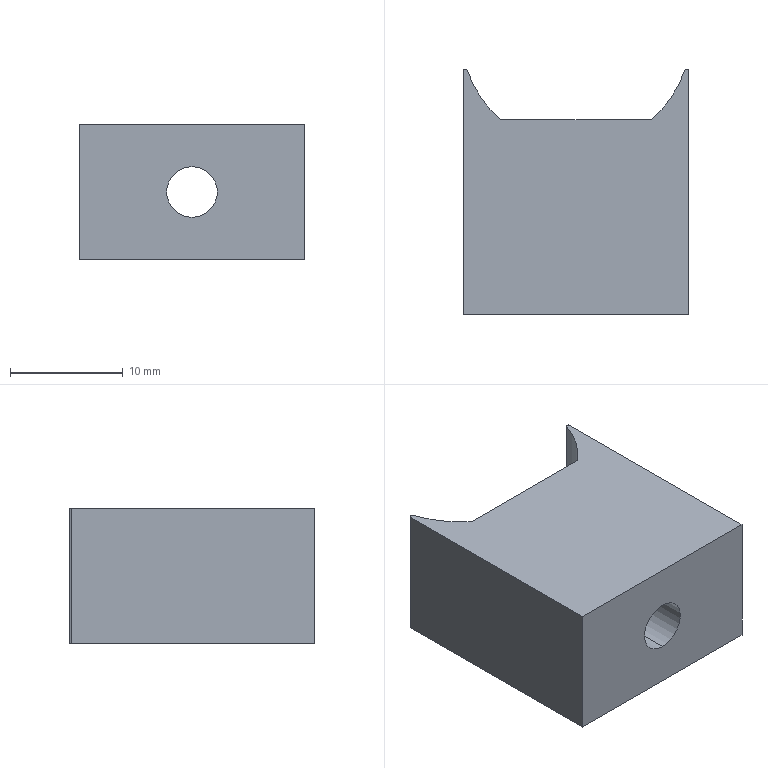Part | STEP file | cylinder positioning fork | 1 solid | 17 faces | box 20 x 21.799 x 12 mm | volume 3903 mm3 | cylinder 10 | plane 7 | commonest cylinder face diameters 0.4 x4 4.5 x2 8 x2 20.4 x2
STEP:
#1=CARTESIAN_POINT('',(0.,0.,0.));
#2=DIRECTION('',(0.,0.,1.));
#3=DIRECTION('',(1.,0.,0.));
#4=AXIS2_PLACEMENT_3D('',#1,#2,#3);
#5=CARTESIAN_POINT('',(0.,-11.7,10.));
#6=VERTEX_POINT('',#5);
#7=CARTESIAN_POINT('',(0.,-7.7,10.));
#8=VERTEX_POINT('',#7);
#9=CARTESIAN_POINT('',(0.,-7.7,10.));
#10=DIRECTION('',(0.,1.,0.));
#11=VECTOR('',#10,1.);
#12=LINE('',#9,#11);
#13=CARTESIAN_POINT('',(0.,-7.7,6.));
#14=DIRECTION('',(0.,1.,0.));
#15=DIRECTION('',(0.,0.,1.));
#16=AXIS2_PLACEMENT_3D('',#13,#14,#15);
#17=CYLINDRICAL_SURFACE('',#16,4.);
#18=CARTESIAN_POINT('',(6.283,0.));
#19=DIRECTION('',(0.,1.));
#20=VECTOR('',#19,1.);
#21=LINE('',#18,#20);
#22=(GEOMETRIC_REPRESENTATION_CONTEXT(2)PARAMETRIC_REPRESENTATION_CONTEXT()REPRESENTATION_CONTEXT('',''));
#23=DEFINITIONAL_REPRESENTATION('',(#21),#22);
#24=PCURVE('',#17,#23);
#25=CARTESIAN_POINT('',(0.,-7.7,6.));
#26=DIRECTION('',(0.,1.,0.));
#27=DIRECTION('',(0.,0.,1.));
#28=AXIS2_PLACEMENT_3D('',#25,#26,#27);
#29=CYLINDRICAL_SURFACE('',#28,4.);
#30=CARTESIAN_POINT('',(0.,0.));
#31=DIRECTION('',(0.,1.));
#32=VECTOR('',#31,1.);
#33=LINE('',#30,#32);
#34=(GEOMETRIC_REPRESENTATION_CONTEXT(2)PARAMETRIC_REPRESENTATION_CONTEXT()REPRESENTATION_CONTEXT('',''));
#35=DEFINITIONAL_REPRESENTATION('',(#33),#34);
#36=PCURVE('',#29,#35);
#37=SURFACE_CURVE('',#12,(#24,#36),.PCURVE_S1.);
#38=EDGE_CURVE('',#6,#8,#37,.T.);
#39=ORIENTED_EDGE('',*,*,#38,.T.);
#40=CARTESIAN_POINT('',(0.,-7.7,2.));
#41=VERTEX_POINT('',#40);
#42=CARTESIAN_POINT('',(0.,-7.7,6.));
#43=DIRECTION('',(0.,1.,0.));
#44=DIRECTION('',(0.,0.,1.));
#45=AXIS2_PLACEMENT_3D('',#42,#43,#44);
#46=CIRCLE('',#45,4.);
#47=CARTESIAN_POINT('',(0.,0.));
#48=DIRECTION('',(1.,0.));
#49=VECTOR('',#48,1.);
#50=LINE('',#47,#49);
#51=(GEOMETRIC_REPRESENTATION_CONTEXT(2)PARAMETRIC_REPRESENTATION_CONTEXT()REPRESENTATION_CONTEXT('',''));
#52=DEFINITIONAL_REPRESENTATION('',(#50),#51);
#53=PCURVE('',#17,#52);
#54=CARTESIAN_POINT('',(-6.69,-7.7,12.));
#55=DIRECTION('',(0.,-1.,0.));
#56=DIRECTION('',(0.,0.,-1.));
#57=AXIS2_PLACEMENT_3D('',#54,#55,#56);
#58=PLANE('',#57);
#59=CARTESIAN_POINT('',(2.,6.69));
#60=CARTESIAN_POINT('',(2.,13.618));
#61=CARTESIAN_POINT('',(8.,10.154));
#62=CARTESIAN_POINT('',(14.,6.69));
#63=CARTESIAN_POINT('',(8.,3.225));
#64=CARTESIAN_POINT('',(2.,-0.2387));
#65=CARTESIAN_POINT('',(2.,6.69));
#66=(BOUNDED_CURVE()B_SPLINE_CURVE(2,(#59,#60,#61,#62,#63,#64,#65),.UNSPECIFIED.,.T.,.F.)B_SPLINE_CURVE_WITH_KNOTS((1,2,2,2,2,1),(-2.094,0.,2.094,4.189,6.283,8.378),.UNSPECIFIED.)CURVE()GEOMETRIC_REPRESENTATION_ITEM()RATIONAL_B_SPLINE_CURVE((1.,0.5,1.,0.5,1.,0.5,1.))REPRESENTATION_ITEM(''));
#67=(GEOMETRIC_REPRESENTATION_CONTEXT(2)PARAMETRIC_REPRESENTATION_CONTEXT()REPRESENTATION_CONTEXT('',''));
#68=DEFINITIONAL_REPRESENTATION('',(#66),#67);
#69=PCURVE('',#58,#68);
#70=SURFACE_CURVE('',#46,(#53,#69),.PCURVE_S1.);
#71=EDGE_CURVE('',#41,#8,#70,.T.);
#72=ORIENTED_EDGE('',*,*,#71,.F.);
#73=CARTESIAN_POINT('',(0.,-11.7,2.));
#74=VERTEX_POINT('',#73);
#75=CARTESIAN_POINT('',(0.,-7.7,2.));
#76=DIRECTION('',(0.,1.,0.));
#77=VECTOR('',#76,1.);
#78=LINE('',#75,#77);
#79=CARTESIAN_POINT('',(3.142,0.));
#80=DIRECTION('',(0.,1.));
#81=VECTOR('',#80,1.);
#82=LINE('',#79,#81);
#83=(GEOMETRIC_REPRESENTATION_CONTEXT(2)PARAMETRIC_REPRESENTATION_CONTEXT()REPRESENTATION_CONTEXT('',''));
#84=DEFINITIONAL_REPRESENTATION('',(#82),#83);
#85=PCURVE('',#17,#84);
#86=CARTESIAN_POINT('',(3.142,0.));
#87=DIRECTION('',(0.,1.));
#88=VECTOR('',#87,1.);
#89=LINE('',#86,#88);
#90=(GEOMETRIC_REPRESENTATION_CONTEXT(2)PARAMETRIC_REPRESENTATION_CONTEXT()REPRESENTATION_CONTEXT('',''));
#91=DEFINITIONAL_REPRESENTATION('',(#89),#90);
#92=PCURVE('',#29,#91);
#93=SURFACE_CURVE('',#78,(#85,#92),.PCURVE_S1.);
#94=EDGE_CURVE('',#74,#41,#93,.T.);
#95=ORIENTED_EDGE('',*,*,#94,.F.);
#96=CARTESIAN_POINT('',(0.,-11.7,6.));
#97=DIRECTION('',(0.,1.,0.));
#98=DIRECTION('',(0.,0.,1.));
#99=AXIS2_PLACEMENT_3D('',#96,#97,#98);
#100=CIRCLE('',#99,4.);
#101=CARTESIAN_POINT('',(0.,-4.));
#102=DIRECTION('',(1.,0.));
#103=VECTOR('',#102,1.);
#104=LINE('',#101,#103);
#105=(GEOMETRIC_REPRESENTATION_CONTEXT(2)PARAMETRIC_REPRESENTATION_CONTEXT()REPRESENTATION_CONTEXT('',''));
#106=DEFINITIONAL_REPRESENTATION('',(#104),#105);
#107=PCURVE('',#17,#106);
#108=CARTESIAN_POINT('',(2.25,-11.7,6.));
#109=DIRECTION('',(0.,-1.,0.));
#110=DIRECTION('',(0.,0.,-1.));
#111=AXIS2_PLACEMENT_3D('',#108,#109,#110);
#112=PLANE('',#111);
#113=CARTESIAN_POINT('',(-4.,-2.25));
#114=CARTESIAN_POINT('',(-4.,4.678));
#115=CARTESIAN_POINT('',(2.,1.214));
#116=CARTESIAN_POINT('',(8.,-2.25));
#117=CARTESIAN_POINT('',(2.,-5.714));
#118=CARTESIAN_POINT('',(-4.,-9.178));
#119=CARTESIAN_POINT('',(-4.,-2.25));
#120=(BOUNDED_CURVE()B_SPLINE_CURVE(2,(#113,#114,#115,#116,#117,#118,#119),.UNSPECIFIED.,.T.,.F.)B_SPLINE_CURVE_WITH_KNOTS((1,2,2,2,2,1),(-2.094,0.,2.094,4.189,6.283,8.378),.UNSPECIFIED.)CURVE()GEOMETRIC_REPRESENTATION_ITEM()RATIONAL_B_SPLINE_CURVE((1.,0.5,1.,0.5,1.,0.5,1.))REPRESENTATION_ITEM(''));
#121=(GEOMETRIC_REPRESENTATION_CONTEXT(2)PARAMETRIC_REPRESENTATION_CONTEXT()REPRESENTATION_CONTEXT('',''));
#122=DEFINITIONAL_REPRESENTATION('',(#120),#121);
#123=PCURVE('',#112,#122);
#124=SURFACE_CURVE('',#100,(#107,#123),.PCURVE_S1.);
#125=EDGE_CURVE('',#74,#6,#124,.T.);
#126=ORIENTED_EDGE('',*,*,#125,.T.);
#127=EDGE_LOOP('',(#39,#72,#95,#126));
#128=FACE_BOUND('',#127,.F.);
#129=ADVANCED_FACE('',(#128),#17,.F.);
#130=CARTESIAN_POINT('',(0.,-25.,8.25));
#131=VERTEX_POINT('',#130);
#132=CARTESIAN_POINT('',(0.,-11.7,8.25));
#133=VERTEX_POINT('',#132);
#134=CARTESIAN_POINT('',(0.,-7.7,8.25));
#135=DIRECTION('',(0.,1.,0.));
#136=VECTOR('',#135,1.);
#137=LINE('',#134,#136);
#138=CARTESIAN_POINT('',(0.,-7.7,6.));
#139=DIRECTION('',(0.,1.,0.));
#140=DIRECTION('',(0.,0.,1.));
#141=AXIS2_PLACEMENT_3D('',#138,#139,#140);
#142=CYLINDRICAL_SURFACE('',#141,2.25);
#143=CARTESIAN_POINT('',(6.283,0.));
#144=DIRECTION('',(0.,1.));
#145=VECTOR('',#144,1.);
#146=LINE('',#143,#145);
#147=(GEOMETRIC_REPRESENTATION_CONTEXT(2)PARAMETRIC_REPRESENTATION_CONTEXT()REPRESENTATION_CONTEXT('',''));
#148=DEFINITIONAL_REPRESENTATION('',(#146),#147);
#149=PCURVE('',#142,#148);
#150=CARTESIAN_POINT('',(0.,-7.7,6.));
#151=DIRECTION('',(0.,1.,0.));
#152=DIRECTION('',(0.,0.,1.));
#153=AXIS2_PLACEMENT_3D('',#150,#151,#152);
#154=CYLINDRICAL_SURFACE('',#153,2.25);
#155=CARTESIAN_POINT('',(0.,0.));
#156=DIRECTION('',(0.,1.));
#157=VECTOR('',#156,1.);
#158=LINE('',#155,#157);
#159=(GEOMETRIC_REPRESENTATION_CONTEXT(2)PARAMETRIC_REPRESENTATION_CONTEXT()REPRESENTATION_CONTEXT('',''));
#160=DEFINITIONAL_REPRESENTATION('',(#158),#159);
#161=PCURVE('',#154,#160);
#162=SURFACE_CURVE('',#137,(#149,#161),.PCURVE_S1.);
#163=EDGE_CURVE('',#131,#133,#162,.T.);
#164=ORIENTED_EDGE('',*,*,#163,.T.);
#165=CARTESIAN_POINT('',(0.,-11.7,3.75));
#166=VERTEX_POINT('',#165);
#167=CARTESIAN_POINT('',(0.,-11.7,6.));
#168=DIRECTION('',(0.,1.,0.));
#169=DIRECTION('',(0.,0.,1.));
#170=AXIS2_PLACEMENT_3D('',#167,#168,#169);
#171=CIRCLE('',#170,2.25);
#172=CARTESIAN_POINT('',(0.,-4.));
#173=DIRECTION('',(1.,0.));
#174=VECTOR('',#173,1.);
#175=LINE('',#172,#174);
#176=(GEOMETRIC_REPRESENTATION_CONTEXT(2)PARAMETRIC_REPRESENTATION_CONTEXT()REPRESENTATION_CONTEXT('',''));
#177=DEFINITIONAL_REPRESENTATION('',(#175),#176);
#178=PCURVE('',#142,#177);
#179=CARTESIAN_POINT('',(-2.25,-2.25));
#180=CARTESIAN_POINT('',(-2.25,1.647));
#181=CARTESIAN_POINT('',(1.125,-0.3014));
#182=CARTESIAN_POINT('',(4.5,-2.25));
#183=CARTESIAN_POINT('',(1.125,-4.199));
#184=CARTESIAN_POINT('',(-2.25,-6.147));
#185=CARTESIAN_POINT('',(-2.25,-2.25));
#186=(BOUNDED_CURVE()B_SPLINE_CURVE(2,(#179,#180,#181,#182,#183,#184,#185),.UNSPECIFIED.,.T.,.F.)B_SPLINE_CURVE_WITH_KNOTS((1,2,2,2,2,1),(-2.094,0.,2.094,4.189,6.283,8.378),.UNSPECIFIED.)CURVE()GEOMETRIC_REPRESENTATION_ITEM()RATIONAL_B_SPLINE_CURVE((1.,0.5,1.,0.5,1.,0.5,1.))REPRESENTATION_ITEM(''));
#187=(GEOMETRIC_REPRESENTATION_CONTEXT(2)PARAMETRIC_REPRESENTATION_CONTEXT()REPRESENTATION_CONTEXT('',''));
#188=DEFINITIONAL_REPRESENTATION('',(#186),#187);
#189=PCURVE('',#112,#188);
#190=SURFACE_CURVE('',#171,(#178,#189),.PCURVE_S1.);
#191=EDGE_CURVE('',#166,#133,#190,.T.);
#192=ORIENTED_EDGE('',*,*,#191,.F.);
#193=CARTESIAN_POINT('',(0.,-25.,3.75));
#194=VERTEX_POINT('',#193);
#195=CARTESIAN_POINT('',(0.,-7.7,3.75));
#196=DIRECTION('',(0.,1.,0.));
#197=VECTOR('',#196,1.);
#198=LINE('',#195,#197);
#199=CARTESIAN_POINT('',(3.142,0.));
#200=DIRECTION('',(0.,1.));
#201=VECTOR('',#200,1.);
#202=LINE('',#199,#201);
#203=(GEOMETRIC_REPRESENTATION_CONTEXT(2)PARAMETRIC_REPRESENTATION_CONTEXT()REPRESENTATION_CONTEXT('',''));
#204=DEFINITIONAL_REPRESENTATION('',(#202),#203);
#205=PCURVE('',#142,#204);
#206=CARTESIAN_POINT('',(3.142,0.));
#207=DIRECTION('',(0.,1.));
#208=VECTOR('',#207,1.);
#209=LINE('',#206,#208);
#210=(GEOMETRIC_REPRESENTATION_CONTEXT(2)PARAMETRIC_REPRESENTATION_CONTEXT()REPRESENTATION_CONTEXT('',''));
#211=DEFINITIONAL_REPRESENTATION('',(#209),#210);
#212=PCURVE('',#154,#211);
#213=SURFACE_CURVE('',#198,(#205,#212),.PCURVE_S1.);
#214=EDGE_CURVE('',#194,#166,#213,.T.);
#215=ORIENTED_EDGE('',*,*,#214,.F.);
#216=CARTESIAN_POINT('',(0.,-25.,6.));
#217=DIRECTION('',(0.,1.,0.));
#218=DIRECTION('',(0.,0.,1.));
#219=AXIS2_PLACEMENT_3D('',#216,#217,#218);
#220=CIRCLE('',#219,2.25);
#221=CARTESIAN_POINT('',(0.,-17.3));
#222=DIRECTION('',(1.,0.));
#223=VECTOR('',#222,1.);
#224=LINE('',#221,#223);
#225=(GEOMETRIC_REPRESENTATION_CONTEXT(2)PARAMETRIC_REPRESENTATION_CONTEXT()REPRESENTATION_CONTEXT('',''));
#226=DEFINITIONAL_REPRESENTATION('',(#224),#225);
#227=PCURVE('',#142,#226);
#228=CARTESIAN_POINT('',(-10.,-25.,12.));
#229=DIRECTION('',(0.,1.,0.));
#230=DIRECTION('',(0.,0.,1.));
#231=AXIS2_PLACEMENT_3D('',#228,#229,#230);
#232=PLANE('',#231);
#233=CARTESIAN_POINT('',(-6.,10.));
#234=DIRECTION('',(1.,0.));
#235=AXIS2_PLACEMENT_2D('',#233,#234);
#236=CIRCLE('',#235,2.25);
#237=(GEOMETRIC_REPRESENTATION_CONTEXT(2)PARAMETRIC_REPRESENTATION_CONTEXT()REPRESENTATION_CONTEXT('',''));
#238=DEFINITIONAL_REPRESENTATION('',(#236),#237);
#239=PCURVE('',#232,#238);
#240=SURFACE_CURVE('',#220,(#227,#239),.PCURVE_S1.);
#241=EDGE_CURVE('',#194,#131,#240,.T.);
#242=ORIENTED_EDGE('',*,*,#241,.T.);
#243=EDGE_LOOP('',(#164,#192,#215,#242));
#244=FACE_BOUND('',#243,.F.);
#245=ADVANCED_FACE('',(#244),#142,.F.);
#246=CARTESIAN_POINT('',(0.,-25.,6.));
#247=DIRECTION('',(0.,1.,0.));
#248=DIRECTION('',(0.,0.,1.));
#249=AXIS2_PLACEMENT_3D('',#246,#247,#248);
#250=CIRCLE('',#249,2.25);
#251=CARTESIAN_POINT('',(-6.,10.));
#252=DIRECTION('',(1.,0.));
#253=AXIS2_PLACEMENT_2D('',#251,#252);
#254=CIRCLE('',#253,2.25);
#255=(GEOMETRIC_REPRESENTATION_CONTEXT(2)PARAMETRIC_REPRESENTATION_CONTEXT()REPRESENTATION_CONTEXT('',''));
#256=DEFINITIONAL_REPRESENTATION('',(#254),#255);
#257=PCURVE('',#232,#256);
#258=CARTESIAN_POINT('',(0.,-17.3));
#259=DIRECTION('',(1.,0.));
#260=VECTOR('',#259,1.);
#261=LINE('',#258,#260);
#262=(GEOMETRIC_REPRESENTATION_CONTEXT(2)PARAMETRIC_REPRESENTATION_CONTEXT()REPRESENTATION_CONTEXT('',''));
#263=DEFINITIONAL_REPRESENTATION('',(#261),#262);
#264=PCURVE('',#154,#263);
#265=SURFACE_CURVE('',#250,(#257,#264),.PCURVE_S1.);
#266=EDGE_CURVE('',#131,#194,#265,.T.);
#267=ORIENTED_EDGE('',*,*,#266,.T.);
#268=ORIENTED_EDGE('',*,*,#241,.T.);
#269=EDGE_LOOP('',(#267,#268));
#270=FACE_BOUND('',#269,.T.);
#271=CARTESIAN_POINT('',(-10.,-25.,0.));
#272=VERTEX_POINT('',#271);
#273=CARTESIAN_POINT('',(10.,-25.,0.));
#274=VERTEX_POINT('',#273);
#275=CARTESIAN_POINT('',(-10.,-25.,0.));
#276=DIRECTION('',(1.,0.,0.));
#277=VECTOR('',#276,1.);
#278=LINE('',#275,#277);
#279=CARTESIAN_POINT('',(-12.,0.));
#280=DIRECTION('',(0.,1.));
#281=VECTOR('',#280,1.);
#282=LINE('',#279,#281);
#283=(GEOMETRIC_REPRESENTATION_CONTEXT(2)PARAMETRIC_REPRESENTATION_CONTEXT()REPRESENTATION_CONTEXT('',''));
#284=DEFINITIONAL_REPRESENTATION('',(#282),#283);
#285=PCURVE('',#232,#284);
#286=CARTESIAN_POINT('',(0.,0.,0.));
#287=DIRECTION('',(0.,0.,1.));
#288=DIRECTION('',(1.,0.,0.));
#289=AXIS2_PLACEMENT_3D('',#286,#287,#288);
#290=PLANE('',#289);
#291=CARTESIAN_POINT('',(-10.,-25.));
#292=DIRECTION('',(1.,0.));
#293=VECTOR('',#292,1.);
#294=LINE('',#291,#293);
#295=(GEOMETRIC_REPRESENTATION_CONTEXT(2)PARAMETRIC_REPRESENTATION_CONTEXT()REPRESENTATION_CONTEXT('',''));
#296=DEFINITIONAL_REPRESENTATION('',(#294),#295);
#297=PCURVE('',#290,#296);
#298=SURFACE_CURVE('',#278,(#285,#297),.PCURVE_S1.);
#299=EDGE_CURVE('',#272,#274,#298,.T.);
#300=ORIENTED_EDGE('',*,*,#299,.T.);
#301=CARTESIAN_POINT('',(10.,-25.,12.));
#302=VERTEX_POINT('',#301);
#303=CARTESIAN_POINT('',(10.,-25.,12.));
#304=DIRECTION('',(0.,0.,-1.));
#305=VECTOR('',#304,1.);
#306=LINE('',#303,#305);
#307=CARTESIAN_POINT('',(0.,20.));
#308=DIRECTION('',(-1.,0.));
#309=VECTOR('',#308,1.);
#310=LINE('',#307,#309);
#311=(GEOMETRIC_REPRESENTATION_CONTEXT(2)PARAMETRIC_REPRESENTATION_CONTEXT()REPRESENTATION_CONTEXT('',''));
#312=DEFINITIONAL_REPRESENTATION('',(#310),#311);
#313=PCURVE('',#232,#312);
#314=CARTESIAN_POINT('',(10.,-3.2,12.));
#315=DIRECTION('',(-1.,0.,0.));
#316=DIRECTION('',(0.,-1.,0.));
#317=AXIS2_PLACEMENT_3D('',#314,#315,#316);
#318=PLANE('',#317);
#319=CARTESIAN_POINT('',(21.8,0.));
#320=DIRECTION('',(0.,-1.));
#321=VECTOR('',#320,1.);
#322=LINE('',#319,#321);
#323=(GEOMETRIC_REPRESENTATION_CONTEXT(2)PARAMETRIC_REPRESENTATION_CONTEXT()REPRESENTATION_CONTEXT('',''));
#324=DEFINITIONAL_REPRESENTATION('',(#322),#323);
#325=PCURVE('',#318,#324);
#326=SURFACE_CURVE('',#306,(#313,#325),.PCURVE_S1.);
#327=EDGE_CURVE('',#302,#274,#326,.T.);
#328=ORIENTED_EDGE('',*,*,#327,.F.);
#329=CARTESIAN_POINT('',(-10.,-25.,12.));
#330=VERTEX_POINT('',#329);
#331=CARTESIAN_POINT('',(-10.,-25.,12.));
#332=DIRECTION('',(1.,0.,0.));
#333=VECTOR('',#332,1.);
#334=LINE('',#331,#333);
#335=CARTESIAN_POINT('',(0.,0.));
#336=DIRECTION('',(0.,1.));
#337=VECTOR('',#336,1.);
#338=LINE('',#335,#337);
#339=(GEOMETRIC_REPRESENTATION_CONTEXT(2)PARAMETRIC_REPRESENTATION_CONTEXT()REPRESENTATION_CONTEXT('',''));
#340=DEFINITIONAL_REPRESENTATION('',(#338),#339);
#341=PCURVE('',#232,#340);
#342=CARTESIAN_POINT('',(0.,0.,12.));
#343=DIRECTION('',(0.,0.,1.));
#344=DIRECTION('',(1.,0.,0.));
#345=AXIS2_PLACEMENT_3D('',#342,#343,#344);
#346=PLANE('',#345);
#347=CARTESIAN_POINT('',(-10.,-25.));
#348=DIRECTION('',(1.,0.));
#349=VECTOR('',#348,1.);
#350=LINE('',#347,#349);
#351=(GEOMETRIC_REPRESENTATION_CONTEXT(2)PARAMETRIC_REPRESENTATION_CONTEXT()REPRESENTATION_CONTEXT('',''));
#352=DEFINITIONAL_REPRESENTATION('',(#350),#351);
#353=PCURVE('',#346,#352);
#354=SURFACE_CURVE('',#334,(#341,#353),.PCURVE_S1.);
#355=EDGE_CURVE('',#330,#302,#354,.T.);
#356=ORIENTED_EDGE('',*,*,#355,.F.);
#357=CARTESIAN_POINT('',(-10.,-25.,12.));
#358=DIRECTION('',(0.,0.,-1.));
#359=VECTOR('',#358,1.);
#360=LINE('',#357,#359);
#361=CARTESIAN_POINT('',(0.,0.));
#362=DIRECTION('',(-1.,0.));
#363=VECTOR('',#362,1.);
#364=LINE('',#361,#363);
#365=(GEOMETRIC_REPRESENTATION_CONTEXT(2)PARAMETRIC_REPRESENTATION_CONTEXT()REPRESENTATION_CONTEXT('',''));
#366=DEFINITIONAL_REPRESENTATION('',(#364),#365);
#367=PCURVE('',#232,#366);
#368=CARTESIAN_POINT('',(-10.,-3.2,12.));
#369=DIRECTION('',(1.,0.,0.));
#370=DIRECTION('',(0.,1.,0.));
#371=AXIS2_PLACEMENT_3D('',#368,#369,#370);
#372=PLANE('',#371);
#373=CARTESIAN_POINT('',(-21.8,0.));
#374=DIRECTION('',(0.,-1.));
#375=VECTOR('',#374,1.);
#376=LINE('',#373,#375);
#377=(GEOMETRIC_REPRESENTATION_CONTEXT(2)PARAMETRIC_REPRESENTATION_CONTEXT()REPRESENTATION_CONTEXT('',''));
#378=DEFINITIONAL_REPRESENTATION('',(#376),#377);
#379=PCURVE('',#372,#378);
#380=SURFACE_CURVE('',#360,(#367,#379),.PCURVE_S1.);
#381=EDGE_CURVE('',#330,#272,#380,.T.);
#382=ORIENTED_EDGE('',*,*,#381,.T.);
#383=EDGE_LOOP('',(#300,#328,#356,#382));
#384=FACE_BOUND('',#383,.T.);
#385=ADVANCED_FACE('',(#270,#384),#232,.F.);
#386=CARTESIAN_POINT('',(10.,-3.4,0.));
#387=VERTEX_POINT('',#386);
#388=CARTESIAN_POINT('',(10.,-3.2,0.));
#389=DIRECTION('',(0.,1.,0.));
#390=VECTOR('',#389,1.);
#391=LINE('',#388,#390);
#392=CARTESIAN_POINT('',(0.,-12.));
#393=DIRECTION('',(-1.,0.));
#394=VECTOR('',#393,1.);
#395=LINE('',#392,#394);
#396=(GEOMETRIC_REPRESENTATION_CONTEXT(2)PARAMETRIC_REPRESENTATION_CONTEXT()REPRESENTATION_CONTEXT('',''));
#397=DEFINITIONAL_REPRESENTATION('',(#395),#396);
#398=PCURVE('',#318,#397);
#399=CARTESIAN_POINT('',(10.,-3.2));
#400=DIRECTION('',(0.,1.));
#401=VECTOR('',#400,1.);
#402=LINE('',#399,#401);
#403=(GEOMETRIC_REPRESENTATION_CONTEXT(2)PARAMETRIC_REPRESENTATION_CONTEXT()REPRESENTATION_CONTEXT('',''));
#404=DEFINITIONAL_REPRESENTATION('',(#402),#403);
#405=PCURVE('',#290,#404);
#406=SURFACE_CURVE('',#391,(#398,#405),.PCURVE_S1.);
#407=EDGE_CURVE('',#274,#387,#406,.T.);
#408=ORIENTED_EDGE('',*,*,#407,.T.);
#409=CARTESIAN_POINT('',(10.,-3.4,12.));
#410=VERTEX_POINT('',#409);
#411=CARTESIAN_POINT('',(10.,-3.4,12.));
#412=DIRECTION('',(0.,0.,1.));
#413=VECTOR('',#412,1.);
#414=LINE('',#411,#413);
#415=CARTESIAN_POINT('',(0.2,0.));
#416=DIRECTION('',(0.,1.));
#417=VECTOR('',#416,1.);
#418=LINE('',#415,#417);
#419=(GEOMETRIC_REPRESENTATION_CONTEXT(2)PARAMETRIC_REPRESENTATION_CONTEXT()REPRESENTATION_CONTEXT('',''));
#420=DEFINITIONAL_REPRESENTATION('',(#418),#419);
#421=PCURVE('',#318,#420);
#422=CARTESIAN_POINT('',(9.8,-3.4,12.));
#423=DIRECTION('',(0.,0.,-1.));
#424=DIRECTION('',(-1.,0.,0.));
#425=AXIS2_PLACEMENT_3D('',#422,#423,#424);
#426=CYLINDRICAL_SURFACE('',#425,0.2);
#427=CARTESIAN_POINT('',(3.142,0.));
#428=DIRECTION('',(0.,-1.));
#429=VECTOR('',#428,1.);
#430=LINE('',#427,#429);
#431=(GEOMETRIC_REPRESENTATION_CONTEXT(2)PARAMETRIC_REPRESENTATION_CONTEXT()REPRESENTATION_CONTEXT('',''));
#432=DEFINITIONAL_REPRESENTATION('',(#430),#431);
#433=PCURVE('',#426,#432);
#434=SURFACE_CURVE('',#414,(#421,#433),.PCURVE_S1.);
#435=EDGE_CURVE('',#387,#410,#434,.T.);
#436=ORIENTED_EDGE('',*,*,#435,.T.);
#437=CARTESIAN_POINT('',(10.,-3.2,12.));
#438=DIRECTION('',(0.,1.,0.));
#439=VECTOR('',#438,1.);
#440=LINE('',#437,#439);
#441=CARTESIAN_POINT('',(0.,0.));
#442=DIRECTION('',(-1.,0.));
#443=VECTOR('',#442,1.);
#444=LINE('',#441,#443);
#445=(GEOMETRIC_REPRESENTATION_CONTEXT(2)PARAMETRIC_REPRESENTATION_CONTEXT()REPRESENTATION_CONTEXT('',''));
#446=DEFINITIONAL_REPRESENTATION('',(#444),#445);
#447=PCURVE('',#318,#446);
#448=CARTESIAN_POINT('',(10.,-3.2));
#449=DIRECTION('',(0.,1.));
#450=VECTOR('',#449,1.);
#451=LINE('',#448,#450);
#452=(GEOMETRIC_REPRESENTATION_CONTEXT(2)PARAMETRIC_REPRESENTATION_CONTEXT()REPRESENTATION_CONTEXT('',''));
#453=DEFINITIONAL_REPRESENTATION('',(#451),#452);
#454=PCURVE('',#346,#453);
#455=SURFACE_CURVE('',#440,(#447,#454),.PCURVE_S1.);
#456=EDGE_CURVE('',#302,#410,#455,.T.);
#457=ORIENTED_EDGE('',*,*,#456,.F.);
#458=ORIENTED_EDGE('',*,*,#327,.T.);
#459=EDGE_LOOP('',(#408,#436,#457,#458));
#460=FACE_BOUND('',#459,.T.);
#461=ADVANCED_FACE('',(#460),#318,.F.);
#462=CARTESIAN_POINT('',(6.69,-7.7,12.));
#463=VERTEX_POINT('',#462);
#464=CARTESIAN_POINT('',(6.69,-7.7,0.));
#465=VERTEX_POINT('',#464);
#466=CARTESIAN_POINT('',(6.69,-7.7,12.));
#467=DIRECTION('',(0.,0.,-1.));
#468=VECTOR('',#467,1.);
#469=LINE('',#466,#468);
#470=CARTESIAN_POINT('',(0.,0.,12.));
#471=DIRECTION('',(0.,0.,-1.));
#472=DIRECTION('',(-1.,0.,0.));
#473=AXIS2_PLACEMENT_3D('',#470,#471,#472);
#474=CYLINDRICAL_SURFACE('',#473,10.2);
#475=CARTESIAN_POINT('',(3.997,0.));
#476=DIRECTION('',(0.,1.));
#477=VECTOR('',#476,1.);
#478=LINE('',#475,#477);
#479=(GEOMETRIC_REPRESENTATION_CONTEXT(2)PARAMETRIC_REPRESENTATION_CONTEXT()REPRESENTATION_CONTEXT('',''));
#480=DEFINITIONAL_REPRESENTATION('',(#478),#479);
#481=PCURVE('',#474,#480);
#482=CARTESIAN_POINT('',(0.,13.379));
#483=DIRECTION('',(1.,0.));
#484=VECTOR('',#483,1.);
#485=LINE('',#482,#484);
#486=(GEOMETRIC_REPRESENTATION_CONTEXT(2)PARAMETRIC_REPRESENTATION_CONTEXT()REPRESENTATION_CONTEXT('',''));
#487=DEFINITIONAL_REPRESENTATION('',(#485),#486);
#488=PCURVE('',#58,#487);
#489=SURFACE_CURVE('',#469,(#481,#488),.PCURVE_S1.);
#490=EDGE_CURVE('',#463,#465,#489,.T.);
#491=ORIENTED_EDGE('',*,*,#490,.T.);
#492=CARTESIAN_POINT('',(9.64,-3.335,0.));
#493=VERTEX_POINT('',#492);
#494=CARTESIAN_POINT('',(0.,0.,0.));
#495=DIRECTION('',(0.,0.,-1.));
#496=DIRECTION('',(1.,0.,0.));
#497=AXIS2_PLACEMENT_3D('',#494,#495,#496);
#498=CIRCLE('',#497,10.2);
#499=CARTESIAN_POINT('',(3.142,12.));
#500=DIRECTION('',(1.,0.));
#501=VECTOR('',#500,1.);
#502=LINE('',#499,#501);
#503=(GEOMETRIC_REPRESENTATION_CONTEXT(2)PARAMETRIC_REPRESENTATION_CONTEXT()REPRESENTATION_CONTEXT('',''));
#504=DEFINITIONAL_REPRESENTATION('',(#502),#503);
#505=PCURVE('',#474,#504);
#506=CARTESIAN_POINT('',(10.2,0.));
#507=CARTESIAN_POINT('',(10.2,-17.667));
#508=CARTESIAN_POINT('',(-5.1,-8.833));
#509=CARTESIAN_POINT('',(-20.4,0.));
#510=CARTESIAN_POINT('',(-5.1,8.833));
#511=CARTESIAN_POINT('',(10.2,17.667));
#512=CARTESIAN_POINT('',(10.2,0.));
#513=(BOUNDED_CURVE()B_SPLINE_CURVE(2,(#506,#507,#508,#509,#510,#511,#512),.UNSPECIFIED.,.T.,.F.)B_SPLINE_CURVE_WITH_KNOTS((1,2,2,2,2,1),(-2.094,0.,2.094,4.189,6.283,8.378),.UNSPECIFIED.)CURVE()GEOMETRIC_REPRESENTATION_ITEM()RATIONAL_B_SPLINE_CURVE((1.,0.5,1.,0.5,1.,0.5,1.))REPRESENTATION_ITEM(''));
#514=(GEOMETRIC_REPRESENTATION_CONTEXT(2)PARAMETRIC_REPRESENTATION_CONTEXT()REPRESENTATION_CONTEXT('',''));
#515=DEFINITIONAL_REPRESENTATION('',(#513),#514);
#516=PCURVE('',#290,#515);
#517=SURFACE_CURVE('',#498,(#505,#516),.PCURVE_S1.);
#518=EDGE_CURVE('',#493,#465,#517,.T.);
#519=ORIENTED_EDGE('',*,*,#518,.F.);
#520=CARTESIAN_POINT('',(9.64,-3.335,12.));
#521=VERTEX_POINT('',#520);
#522=CARTESIAN_POINT('',(9.64,-3.335,12.));
#523=DIRECTION('',(0.,0.,-1.));
#524=VECTOR('',#523,1.);
#525=LINE('',#522,#524);
#526=CARTESIAN_POINT('',(3.475,0.));
#527=DIRECTION('',(0.,1.));
#528=VECTOR('',#527,1.);
#529=LINE('',#526,#528);
#530=(GEOMETRIC_REPRESENTATION_CONTEXT(2)PARAMETRIC_REPRESENTATION_CONTEXT()REPRESENTATION_CONTEXT('',''));
#531=DEFINITIONAL_REPRESENTATION('',(#529),#530);
#532=PCURVE('',#474,#531);
#533=CARTESIAN_POINT('',(9.829,-3.4,12.));
#534=DIRECTION('',(0.,0.,-1.));
#535=DIRECTION('',(-1.,0.,0.));
#536=AXIS2_PLACEMENT_3D('',#533,#534,#535);
#537=CYLINDRICAL_SURFACE('',#536,0.2);
#538=CARTESIAN_POINT('',(0.333,0.));
#539=DIRECTION('',(0.,1.));
#540=VECTOR('',#539,1.);
#541=LINE('',#538,#540);
#542=(GEOMETRIC_REPRESENTATION_CONTEXT(2)PARAMETRIC_REPRESENTATION_CONTEXT()REPRESENTATION_CONTEXT('',''));
#543=DEFINITIONAL_REPRESENTATION('',(#541),#542);
#544=PCURVE('',#537,#543);
#545=SURFACE_CURVE('',#525,(#532,#544),.PCURVE_S1.);
#546=EDGE_CURVE('',#521,#493,#545,.T.);
#547=ORIENTED_EDGE('',*,*,#546,.F.);
#548=CARTESIAN_POINT('',(0.,0.,12.));
#549=DIRECTION('',(0.,0.,-1.));
#550=DIRECTION('',(1.,0.,0.));
#551=AXIS2_PLACEMENT_3D('',#548,#549,#550);
#552=CIRCLE('',#551,10.2);
#553=CARTESIAN_POINT('',(3.142,0.));
#554=DIRECTION('',(1.,0.));
#555=VECTOR('',#554,1.);
#556=LINE('',#553,#555);
#557=(GEOMETRIC_REPRESENTATION_CONTEXT(2)PARAMETRIC_REPRESENTATION_CONTEXT()REPRESENTATION_CONTEXT('',''));
#558=DEFINITIONAL_REPRESENTATION('',(#556),#557);
#559=PCURVE('',#474,#558);
#560=CARTESIAN_POINT('',(10.2,0.));
#561=CARTESIAN_POINT('',(10.2,-17.667));
#562=CARTESIAN_POINT('',(-5.1,-8.833));
#563=CARTESIAN_POINT('',(-20.4,0.));
#564=CARTESIAN_POINT('',(-5.1,8.833));
#565=CARTESIAN_POINT('',(10.2,17.667));
#566=CARTESIAN_POINT('',(10.2,0.));
#567=(BOUNDED_CURVE()B_SPLINE_CURVE(2,(#560,#561,#562,#563,#564,#565,#566),.UNSPECIFIED.,.T.,.F.)B_SPLINE_CURVE_WITH_KNOTS((1,2,2,2,2,1),(-2.094,0.,2.094,4.189,6.283,8.378),.UNSPECIFIED.)CURVE()GEOMETRIC_REPRESENTATION_ITEM()RATIONAL_B_SPLINE_CURVE((1.,0.5,1.,0.5,1.,0.5,1.))REPRESENTATION_ITEM(''));
#568=(GEOMETRIC_REPRESENTATION_CONTEXT(2)PARAMETRIC_REPRESENTATION_CONTEXT()REPRESENTATION_CONTEXT('',''));
#569=DEFINITIONAL_REPRESENTATION('',(#567),#568);
#570=PCURVE('',#346,#569);
#571=SURFACE_CURVE('',#552,(#559,#570),.PCURVE_S1.);
#572=EDGE_CURVE('',#521,#463,#571,.T.);
#573=ORIENTED_EDGE('',*,*,#572,.T.);
#574=EDGE_LOOP('',(#491,#519,#547,#573));
#575=FACE_BOUND('',#574,.F.);
#576=ADVANCED_FACE('',(#575),#474,.F.);
#577=CARTESIAN_POINT('',(0.,-7.7,6.));
#578=DIRECTION('',(0.,1.,0.));
#579=DIRECTION('',(0.,0.,1.));
#580=AXIS2_PLACEMENT_3D('',#577,#578,#579);
#581=CIRCLE('',#580,4.);
#582=CARTESIAN_POINT('',(2.,6.69));
#583=CARTESIAN_POINT('',(2.,13.618));
#584=CARTESIAN_POINT('',(8.,10.154));
#585=CARTESIAN_POINT('',(14.,6.69));
#586=CARTESIAN_POINT('',(8.,3.225));
#587=CARTESIAN_POINT('',(2.,-0.2387));
#588=CARTESIAN_POINT('',(2.,6.69));
#589=(BOUNDED_CURVE()B_SPLINE_CURVE(2,(#582,#583,#584,#585,#586,#587,#588),.UNSPECIFIED.,.T.,.F.)B_SPLINE_CURVE_WITH_KNOTS((1,2,2,2,2,1),(-2.094,0.,2.094,4.189,6.283,8.378),.UNSPECIFIED.)CURVE()GEOMETRIC_REPRESENTATION_ITEM()RATIONAL_B_SPLINE_CURVE((1.,0.5,1.,0.5,1.,0.5,1.))REPRESENTATION_ITEM(''));
#590=(GEOMETRIC_REPRESENTATION_CONTEXT(2)PARAMETRIC_REPRESENTATION_CONTEXT()REPRESENTATION_CONTEXT('',''));
#591=DEFINITIONAL_REPRESENTATION('',(#589),#590);
#592=PCURVE('',#58,#591);
#593=CARTESIAN_POINT('',(0.,0.));
#594=DIRECTION('',(1.,0.));
#595=VECTOR('',#594,1.);
#596=LINE('',#593,#595);
#597=(GEOMETRIC_REPRESENTATION_CONTEXT(2)PARAMETRIC_REPRESENTATION_CONTEXT()REPRESENTATION_CONTEXT('',''));
#598=DEFINITIONAL_REPRESENTATION('',(#596),#597);
#599=PCURVE('',#29,#598);
#600=SURFACE_CURVE('',#581,(#592,#599),.PCURVE_S1.);
#601=EDGE_CURVE('',#8,#41,#600,.T.);
#602=ORIENTED_EDGE('',*,*,#601,.F.);
#603=ORIENTED_EDGE('',*,*,#71,.F.);
#604=EDGE_LOOP('',(#602,#603));
#605=FACE_BOUND('',#604,.T.);
#606=CARTESIAN_POINT('',(-6.69,-7.7,0.));
#607=VERTEX_POINT('',#606);
#608=CARTESIAN_POINT('',(-6.69,-7.7,0.));
#609=DIRECTION('',(-1.,0.,0.));
#610=VECTOR('',#609,1.);
#611=LINE('',#608,#610);
#612=CARTESIAN_POINT('',(12.,0.));
#613=DIRECTION('',(0.,-1.));
#614=VECTOR('',#613,1.);
#615=LINE('',#612,#614);
#616=(GEOMETRIC_REPRESENTATION_CONTEXT(2)PARAMETRIC_REPRESENTATION_CONTEXT()REPRESENTATION_CONTEXT('',''));
#617=DEFINITIONAL_REPRESENTATION('',(#615),#616);
#618=PCURVE('',#58,#617);
#619=CARTESIAN_POINT('',(-6.69,-7.7));
#620=DIRECTION('',(-1.,0.));
#621=VECTOR('',#620,1.);
#622=LINE('',#619,#621);
#623=(GEOMETRIC_REPRESENTATION_CONTEXT(2)PARAMETRIC_REPRESENTATION_CONTEXT()REPRESENTATION_CONTEXT('',''));
#624=DEFINITIONAL_REPRESENTATION('',(#622),#623);
#625=PCURVE('',#290,#624);
#626=SURFACE_CURVE('',#611,(#618,#625),.PCURVE_S1.);
#627=EDGE_CURVE('',#465,#607,#626,.T.);
#628=ORIENTED_EDGE('',*,*,#627,.T.);
#629=CARTESIAN_POINT('',(-6.69,-7.7,12.));
#630=VERTEX_POINT('',#629);
#631=CARTESIAN_POINT('',(-6.69,-7.7,12.));
#632=DIRECTION('',(0.,0.,-1.));
#633=VECTOR('',#632,1.);
#634=LINE('',#631,#633);
#635=CARTESIAN_POINT('',(0.,0.));
#636=DIRECTION('',(1.,0.));
#637=VECTOR('',#636,1.);
#638=LINE('',#635,#637);
#639=(GEOMETRIC_REPRESENTATION_CONTEXT(2)PARAMETRIC_REPRESENTATION_CONTEXT()REPRESENTATION_CONTEXT('',''));
#640=DEFINITIONAL_REPRESENTATION('',(#638),#639);
#641=PCURVE('',#58,#640);
#642=CARTESIAN_POINT('',(0.,0.,12.));
#643=DIRECTION('',(0.,0.,-1.));
#644=DIRECTION('',(-1.,0.,0.));
#645=AXIS2_PLACEMENT_3D('',#642,#643,#644);
#646=CYLINDRICAL_SURFACE('',#645,10.2);
#647=CARTESIAN_POINT('',(5.428,0.));
#648=DIRECTION('',(0.,1.));
#649=VECTOR('',#648,1.);
#650=LINE('',#647,#649);
#651=(GEOMETRIC_REPRESENTATION_CONTEXT(2)PARAMETRIC_REPRESENTATION_CONTEXT()REPRESENTATION_CONTEXT('',''));
#652=DEFINITIONAL_REPRESENTATION('',(#650),#651);
#653=PCURVE('',#646,#652);
#654=SURFACE_CURVE('',#634,(#641,#653),.PCURVE_S1.);
#655=EDGE_CURVE('',#630,#607,#654,.T.);
#656=ORIENTED_EDGE('',*,*,#655,.F.);
#657=CARTESIAN_POINT('',(-6.69,-7.7,12.));
#658=DIRECTION('',(-1.,0.,0.));
#659=VECTOR('',#658,1.);
#660=LINE('',#657,#659);
#661=CARTESIAN_POINT('',(0.,0.));
#662=DIRECTION('',(0.,-1.));
#663=VECTOR('',#662,1.);
#664=LINE('',#661,#663);
#665=(GEOMETRIC_REPRESENTATION_CONTEXT(2)PARAMETRIC_REPRESENTATION_CONTEXT()REPRESENTATION_CONTEXT('',''));
#666=DEFINITIONAL_REPRESENTATION('',(#664),#665);
#667=PCURVE('',#58,#666);
#668=CARTESIAN_POINT('',(-6.69,-7.7));
#669=DIRECTION('',(-1.,0.));
#670=VECTOR('',#669,1.);
#671=LINE('',#668,#670);
#672=(GEOMETRIC_REPRESENTATION_CONTEXT(2)PARAMETRIC_REPRESENTATION_CONTEXT()REPRESENTATION_CONTEXT('',''));
#673=DEFINITIONAL_REPRESENTATION('',(#671),#672);
#674=PCURVE('',#346,#673);
#675=SURFACE_CURVE('',#660,(#667,#674),.PCURVE_S1.);
#676=EDGE_CURVE('',#463,#630,#675,.T.);
#677=ORIENTED_EDGE('',*,*,#676,.F.);
#678=ORIENTED_EDGE('',*,*,#490,.T.);
#679=EDGE_LOOP('',(#628,#656,#677,#678));
#680=FACE_BOUND('',#679,.T.);
#681=ADVANCED_FACE('',(#605,#680),#58,.F.);
#682=ORIENTED_EDGE('',*,*,#655,.F.);
#683=CARTESIAN_POINT('',(-9.64,-3.335,12.));
#684=VERTEX_POINT('',#683);
#685=CARTESIAN_POINT('',(0.,0.,12.));
#686=DIRECTION('',(0.,0.,-1.));
#687=DIRECTION('',(1.,0.,0.));
#688=AXIS2_PLACEMENT_3D('',#685,#686,#687);
#689=CIRCLE('',#688,10.2);
#690=CARTESIAN_POINT('',(3.142,0.));
#691=DIRECTION('',(1.,0.));
#692=VECTOR('',#691,1.);
#693=LINE('',#690,#692);
#694=(GEOMETRIC_REPRESENTATION_CONTEXT(2)PARAMETRIC_REPRESENTATION_CONTEXT()REPRESENTATION_CONTEXT('',''));
#695=DEFINITIONAL_REPRESENTATION('',(#693),#694);
#696=PCURVE('',#646,#695);
#697=CARTESIAN_POINT('',(10.2,0.));
#698=CARTESIAN_POINT('',(10.2,-17.667));
#699=CARTESIAN_POINT('',(-5.1,-8.833));
#700=CARTESIAN_POINT('',(-20.4,0.));
#701=CARTESIAN_POINT('',(-5.1,8.833));
#702=CARTESIAN_POINT('',(10.2,17.667));
#703=CARTESIAN_POINT('',(10.2,0.));
#704=(BOUNDED_CURVE()B_SPLINE_CURVE(2,(#697,#698,#699,#700,#701,#702,#703),.UNSPECIFIED.,.T.,.F.)B_SPLINE_CURVE_WITH_KNOTS((1,2,2,2,2,1),(-2.094,0.,2.094,4.189,6.283,8.378),.UNSPECIFIED.)CURVE()GEOMETRIC_REPRESENTATION_ITEM()RATIONAL_B_SPLINE_CURVE((1.,0.5,1.,0.5,1.,0.5,1.))REPRESENTATION_ITEM(''));
#705=(GEOMETRIC_REPRESENTATION_CONTEXT(2)PARAMETRIC_REPRESENTATION_CONTEXT()REPRESENTATION_CONTEXT('',''));
#706=DEFINITIONAL_REPRESENTATION('',(#704),#705);
#707=PCURVE('',#346,#706);
#708=SURFACE_CURVE('',#689,(#696,#707),.PCURVE_S1.);
#709=EDGE_CURVE('',#630,#684,#708,.T.);
#710=ORIENTED_EDGE('',*,*,#709,.T.);
#711=CARTESIAN_POINT('',(-9.64,-3.335,0.));
#712=VERTEX_POINT('',#711);
#713=CARTESIAN_POINT('',(-9.64,-3.335,12.));
#714=DIRECTION('',(0.,0.,1.));
#715=VECTOR('',#714,1.);
#716=LINE('',#713,#715);
#717=CARTESIAN_POINT('',(5.95,0.));
#718=DIRECTION('',(0.,-1.));
#719=VECTOR('',#718,1.);
#720=LINE('',#717,#719);
#721=(GEOMETRIC_REPRESENTATION_CONTEXT(2)PARAMETRIC_REPRESENTATION_CONTEXT()REPRESENTATION_CONTEXT('',''));
#722=DEFINITIONAL_REPRESENTATION('',(#720),#721);
#723=PCURVE('',#646,#722);
#724=CARTESIAN_POINT('',(-9.829,-3.4,12.));
#725=DIRECTION('',(0.,0.,-1.));
#726=DIRECTION('',(-1.,0.,0.));
#727=AXIS2_PLACEMENT_3D('',#724,#725,#726);
#728=CYLINDRICAL_SURFACE('',#727,0.2);
#729=CARTESIAN_POINT('',(2.809,0.));
#730=DIRECTION('',(0.,-1.));
#731=VECTOR('',#730,1.);
#732=LINE('',#729,#731);
#733=(GEOMETRIC_REPRESENTATION_CONTEXT(2)PARAMETRIC_REPRESENTATION_CONTEXT()REPRESENTATION_CONTEXT('',''));
#734=DEFINITIONAL_REPRESENTATION('',(#732),#733);
#735=PCURVE('',#728,#734);
#736=SURFACE_CURVE('',#716,(#723,#735),.PCURVE_S1.);
#737=EDGE_CURVE('',#712,#684,#736,.T.);
#738=ORIENTED_EDGE('',*,*,#737,.F.);
#739=CARTESIAN_POINT('',(0.,0.,0.));
#740=DIRECTION('',(0.,0.,-1.));
#741=DIRECTION('',(1.,0.,0.));
#742=AXIS2_PLACEMENT_3D('',#739,#740,#741);
#743=CIRCLE('',#742,10.2);
#744=CARTESIAN_POINT('',(3.142,12.));
#745=DIRECTION('',(1.,0.));
#746=VECTOR('',#745,1.);
#747=LINE('',#744,#746);
#748=(GEOMETRIC_REPRESENTATION_CONTEXT(2)PARAMETRIC_REPRESENTATION_CONTEXT()REPRESENTATION_CONTEXT('',''));
#749=DEFINITIONAL_REPRESENTATION('',(#747),#748);
#750=PCURVE('',#646,#749);
#751=CARTESIAN_POINT('',(10.2,0.));
#752=CARTESIAN_POINT('',(10.2,-17.667));
#753=CARTESIAN_POINT('',(-5.1,-8.833));
#754=CARTESIAN_POINT('',(-20.4,0.));
#755=CARTESIAN_POINT('',(-5.1,8.833));
#756=CARTESIAN_POINT('',(10.2,17.667));
#757=CARTESIAN_POINT('',(10.2,0.));
#758=(BOUNDED_CURVE()B_SPLINE_CURVE(2,(#751,#752,#753,#754,#755,#756,#757),.UNSPECIFIED.,.T.,.F.)B_SPLINE_CURVE_WITH_KNOTS((1,2,2,2,2,1),(-2.094,0.,2.094,4.189,6.283,8.378),.UNSPECIFIED.)CURVE()GEOMETRIC_REPRESENTATION_ITEM()RATIONAL_B_SPLINE_CURVE((1.,0.5,1.,0.5,1.,0.5,1.))REPRESENTATION_ITEM(''));
#759=(GEOMETRIC_REPRESENTATION_CONTEXT(2)PARAMETRIC_REPRESENTATION_CONTEXT()REPRESENTATION_CONTEXT('',''));
#760=DEFINITIONAL_REPRESENTATION('',(#758),#759);
#761=PCURVE('',#290,#760);
#762=SURFACE_CURVE('',#743,(#750,#761),.PCURVE_S1.);
#763=EDGE_CURVE('',#607,#712,#762,.T.);
#764=ORIENTED_EDGE('',*,*,#763,.F.);
#765=EDGE_LOOP('',(#682,#710,#738,#764));
#766=FACE_BOUND('',#765,.F.);
#767=ADVANCED_FACE('',(#766),#646,.F.);
#768=CARTESIAN_POINT('',(-10.,-3.4,12.));
#769=VERTEX_POINT('',#768);
#770=CARTESIAN_POINT('',(-10.,-3.2,12.));
#771=DIRECTION('',(0.,-1.,0.));
#772=VECTOR('',#771,1.);
#773=LINE('',#770,#772);
#774=CARTESIAN_POINT('',(0.,0.));
#775=DIRECTION('',(-1.,0.));
#776=VECTOR('',#775,1.);
#777=LINE('',#774,#776);
#778=(GEOMETRIC_REPRESENTATION_CONTEXT(2)PARAMETRIC_REPRESENTATION_CONTEXT()REPRESENTATION_CONTEXT('',''));
#779=DEFINITIONAL_REPRESENTATION('',(#777),#778);
#780=PCURVE('',#372,#779);
#781=CARTESIAN_POINT('',(-10.,-3.2));
#782=DIRECTION('',(0.,-1.));
#783=VECTOR('',#782,1.);
#784=LINE('',#781,#783);
#785=(GEOMETRIC_REPRESENTATION_CONTEXT(2)PARAMETRIC_REPRESENTATION_CONTEXT()REPRESENTATION_CONTEXT('',''));
#786=DEFINITIONAL_REPRESENTATION('',(#784),#785);
#787=PCURVE('',#346,#786);
#788=SURFACE_CURVE('',#773,(#780,#787),.PCURVE_S1.);
#789=EDGE_CURVE('',#769,#330,#788,.T.);
#790=ORIENTED_EDGE('',*,*,#789,.F.);
#791=CARTESIAN_POINT('',(-10.,-3.4,0.));
#792=VERTEX_POINT('',#791);
#793=CARTESIAN_POINT('',(-10.,-3.4,12.));
#794=DIRECTION('',(0.,0.,-1.));
#795=VECTOR('',#794,1.);
#796=LINE('',#793,#795);
#797=CARTESIAN_POINT('',(-0.2,0.));
#798=DIRECTION('',(0.,-1.));
#799=VECTOR('',#798,1.);
#800=LINE('',#797,#799);
#801=(GEOMETRIC_REPRESENTATION_CONTEXT(2)PARAMETRIC_REPRESENTATION_CONTEXT()REPRESENTATION_CONTEXT('',''));
#802=DEFINITIONAL_REPRESENTATION('',(#800),#801);
#803=PCURVE('',#372,#802);
#804=CARTESIAN_POINT('',(-9.8,-3.4,12.));
#805=DIRECTION('',(0.,0.,-1.));
#806=DIRECTION('',(-1.,0.,0.));
#807=AXIS2_PLACEMENT_3D('',#804,#805,#806);
#808=CYLINDRICAL_SURFACE('',#807,0.2);
#809=CARTESIAN_POINT('',(0.,0.));
#810=DIRECTION('',(0.,1.));
#811=VECTOR('',#810,1.);
#812=LINE('',#809,#811);
#813=(GEOMETRIC_REPRESENTATION_CONTEXT(2)PARAMETRIC_REPRESENTATION_CONTEXT()REPRESENTATION_CONTEXT('',''));
#814=DEFINITIONAL_REPRESENTATION('',(#812),#813);
#815=PCURVE('',#808,#814);
#816=SURFACE_CURVE('',#796,(#803,#815),.PCURVE_S1.);
#817=EDGE_CURVE('',#769,#792,#816,.T.);
#818=ORIENTED_EDGE('',*,*,#817,.T.);
#819=CARTESIAN_POINT('',(-10.,-3.2,0.));
#820=DIRECTION('',(0.,-1.,0.));
#821=VECTOR('',#820,1.);
#822=LINE('',#819,#821);
#823=CARTESIAN_POINT('',(0.,-12.));
#824=DIRECTION('',(-1.,0.));
#825=VECTOR('',#824,1.);
#826=LINE('',#823,#825);
#827=(GEOMETRIC_REPRESENTATION_CONTEXT(2)PARAMETRIC_REPRESENTATION_CONTEXT()REPRESENTATION_CONTEXT('',''));
#828=DEFINITIONAL_REPRESENTATION('',(#826),#827);
#829=PCURVE('',#372,#828);
#830=CARTESIAN_POINT('',(-10.,-3.2));
#831=DIRECTION('',(0.,-1.));
#832=VECTOR('',#831,1.);
#833=LINE('',#830,#832);
#834=(GEOMETRIC_REPRESENTATION_CONTEXT(2)PARAMETRIC_REPRESENTATION_CONTEXT()REPRESENTATION_CONTEXT('',''));
#835=DEFINITIONAL_REPRESENTATION('',(#833),#834);
#836=PCURVE('',#290,#835);
#837=SURFACE_CURVE('',#822,(#829,#836),.PCURVE_S1.);
#838=EDGE_CURVE('',#792,#272,#837,.T.);
#839=ORIENTED_EDGE('',*,*,#838,.T.);
#840=ORIENTED_EDGE('',*,*,#381,.F.);
#841=EDGE_LOOP('',(#790,#818,#839,#840));
#842=FACE_BOUND('',#841,.T.);
#843=ADVANCED_FACE('',(#842),#372,.F.);
#844=CARTESIAN_POINT('',(-9.814,-3.201,12.));
#845=VERTEX_POINT('',#844);
#846=CARTESIAN_POINT('',(-9.829,-3.4,12.));
#847=DIRECTION('',(0.,0.,1.));
#848=DIRECTION('',(1.,0.,0.));
#849=AXIS2_PLACEMENT_3D('',#846,#847,#848);
#850=CIRCLE('',#849,0.2);
#851=CARTESIAN_POINT('',(-9.829,-3.4));
#852=DIRECTION('',(1.,0.));
#853=AXIS2_PLACEMENT_2D('',#851,#852);
#854=CIRCLE('',#853,0.2);
#855=(GEOMETRIC_REPRESENTATION_CONTEXT(2)PARAMETRIC_REPRESENTATION_CONTEXT()REPRESENTATION_CONTEXT('',''));
#856=DEFINITIONAL_REPRESENTATION('',(#854),#855);
#857=PCURVE('',#346,#856);
#858=CARTESIAN_POINT('',(3.142,0.));
#859=DIRECTION('',(-1.,0.));
#860=VECTOR('',#859,1.);
#861=LINE('',#858,#860);
#862=(GEOMETRIC_REPRESENTATION_CONTEXT(2)PARAMETRIC_REPRESENTATION_CONTEXT()REPRESENTATION_CONTEXT('',''));
#863=DEFINITIONAL_REPRESENTATION('',(#861),#862);
#864=PCURVE('',#728,#863);
#865=SURFACE_CURVE('',#850,(#857,#864),.PCURVE_S1.);
#866=EDGE_CURVE('',#684,#845,#865,.T.);
#867=ORIENTED_EDGE('',*,*,#866,.T.);
#868=CARTESIAN_POINT('',(-9.8,-3.4,12.));
#869=DIRECTION('',(0.,0.,1.));
#870=DIRECTION('',(1.,0.,0.));
#871=AXIS2_PLACEMENT_3D('',#868,#869,#870);
#872=CIRCLE('',#871,0.2);
#873=CARTESIAN_POINT('',(-9.8,-3.4));
#874=DIRECTION('',(1.,0.));
#875=AXIS2_PLACEMENT_2D('',#873,#874);
#876=CIRCLE('',#875,0.2);
#877=(GEOMETRIC_REPRESENTATION_CONTEXT(2)PARAMETRIC_REPRESENTATION_CONTEXT()REPRESENTATION_CONTEXT('',''));
#878=DEFINITIONAL_REPRESENTATION('',(#876),#877);
#879=PCURVE('',#346,#878);
#880=CARTESIAN_POINT('',(3.142,0.));
#881=DIRECTION('',(-1.,0.));
#882=VECTOR('',#881,1.);
#883=LINE('',#880,#882);
#884=(GEOMETRIC_REPRESENTATION_CONTEXT(2)PARAMETRIC_REPRESENTATION_CONTEXT()REPRESENTATION_CONTEXT('',''));
#885=DEFINITIONAL_REPRESENTATION('',(#883),#884);
#886=PCURVE('',#808,#885);
#887=SURFACE_CURVE('',#872,(#879,#886),.PCURVE_S1.);
#888=EDGE_CURVE('',#845,#769,#887,.T.);
#889=ORIENTED_EDGE('',*,*,#888,.T.);
#890=ORIENTED_EDGE('',*,*,#789,.T.);
#891=ORIENTED_EDGE('',*,*,#355,.T.);
#892=ORIENTED_EDGE('',*,*,#456,.T.);
#893=CARTESIAN_POINT('',(9.814,-3.201,12.));
#894=VERTEX_POINT('',#893);
#895=CARTESIAN_POINT('',(9.8,-3.4,12.));
#896=DIRECTION('',(0.,0.,1.));
#897=DIRECTION('',(1.,0.,0.));
#898=AXIS2_PLACEMENT_3D('',#895,#896,#897);
#899=CIRCLE('',#898,0.2);
#900=CARTESIAN_POINT('',(9.8,-3.4));
#901=DIRECTION('',(1.,0.));
#902=AXIS2_PLACEMENT_2D('',#900,#901);
#903=CIRCLE('',#902,0.2);
#904=(GEOMETRIC_REPRESENTATION_CONTEXT(2)PARAMETRIC_REPRESENTATION_CONTEXT()REPRESENTATION_CONTEXT('',''));
#905=DEFINITIONAL_REPRESENTATION('',(#903),#904);
#906=PCURVE('',#346,#905);
#907=CARTESIAN_POINT('',(3.142,0.));
#908=DIRECTION('',(-1.,0.));
#909=VECTOR('',#908,1.);
#910=LINE('',#907,#909);
#911=(GEOMETRIC_REPRESENTATION_CONTEXT(2)PARAMETRIC_REPRESENTATION_CONTEXT()REPRESENTATION_CONTEXT('',''));
#912=DEFINITIONAL_REPRESENTATION('',(#910),#911);
#913=PCURVE('',#426,#912);
#914=SURFACE_CURVE('',#899,(#906,#913),.PCURVE_S1.);
#915=EDGE_CURVE('',#410,#894,#914,.T.);
#916=ORIENTED_EDGE('',*,*,#915,.T.);
#917=CARTESIAN_POINT('',(9.829,-3.4,12.));
#918=DIRECTION('',(0.,0.,1.));
#919=DIRECTION('',(1.,0.,0.));
#920=AXIS2_PLACEMENT_3D('',#917,#918,#919);
#921=CIRCLE('',#920,0.2);
#922=CARTESIAN_POINT('',(9.829,-3.4));
#923=DIRECTION('',(1.,0.));
#924=AXIS2_PLACEMENT_2D('',#922,#923);
#925=CIRCLE('',#924,0.2);
#926=(GEOMETRIC_REPRESENTATION_CONTEXT(2)PARAMETRIC_REPRESENTATION_CONTEXT()REPRESENTATION_CONTEXT('',''));
#927=DEFINITIONAL_REPRESENTATION('',(#925),#926);
#928=PCURVE('',#346,#927);
#929=CARTESIAN_POINT('',(3.142,0.));
#930=DIRECTION('',(-1.,0.));
#931=VECTOR('',#930,1.);
#932=LINE('',#929,#931);
#933=(GEOMETRIC_REPRESENTATION_CONTEXT(2)PARAMETRIC_REPRESENTATION_CONTEXT()REPRESENTATION_CONTEXT('',''));
#934=DEFINITIONAL_REPRESENTATION('',(#932),#933);
#935=PCURVE('',#537,#934);
#936=SURFACE_CURVE('',#921,(#928,#935),.PCURVE_S1.);
#937=EDGE_CURVE('',#894,#521,#936,.T.);
#938=ORIENTED_EDGE('',*,*,#937,.T.);
#939=ORIENTED_EDGE('',*,*,#572,.T.);
#940=ORIENTED_EDGE('',*,*,#676,.T.);
#941=ORIENTED_EDGE('',*,*,#709,.T.);
#942=EDGE_LOOP('',(#867,#889,#890,#891,#892,#916,#938,#939,#940,#941));
#943=FACE_BOUND('',#942,.T.);
#944=ADVANCED_FACE('',(#943),#346,.T.);
#945=ORIENTED_EDGE('',*,*,#838,.F.);
#946=CARTESIAN_POINT('',(-9.814,-3.201,0.));
#947=VERTEX_POINT('',#946);
#948=CARTESIAN_POINT('',(-9.8,-3.4,0.));
#949=DIRECTION('',(0.,0.,-1.));
#950=DIRECTION('',(1.,0.,0.));
#951=AXIS2_PLACEMENT_3D('',#948,#949,#950);
#952=CIRCLE('',#951,0.2);
#953=CARTESIAN_POINT('',(-9.6,-3.4));
#954=CARTESIAN_POINT('',(-9.6,-3.746));
#955=CARTESIAN_POINT('',(-9.9,-3.573));
#956=CARTESIAN_POINT('',(-10.2,-3.4));
#957=CARTESIAN_POINT('',(-9.9,-3.227));
#958=CARTESIAN_POINT('',(-9.6,-3.054));
#959=CARTESIAN_POINT('',(-9.6,-3.4));
#960=(BOUNDED_CURVE()B_SPLINE_CURVE(2,(#953,#954,#955,#956,#957,#958,#959),.UNSPECIFIED.,.T.,.F.)B_SPLINE_CURVE_WITH_KNOTS((1,2,2,2,2,1),(-2.094,0.,2.094,4.189,6.283,8.378),.UNSPECIFIED.)CURVE()GEOMETRIC_REPRESENTATION_ITEM()RATIONAL_B_SPLINE_CURVE((1.,0.5,1.,0.5,1.,0.5,1.))REPRESENTATION_ITEM(''));
#961=(GEOMETRIC_REPRESENTATION_CONTEXT(2)PARAMETRIC_REPRESENTATION_CONTEXT()REPRESENTATION_CONTEXT('',''));
#962=DEFINITIONAL_REPRESENTATION('',(#960),#961);
#963=PCURVE('',#290,#962);
#964=CARTESIAN_POINT('',(-3.142,12.));
#965=DIRECTION('',(1.,0.));
#966=VECTOR('',#965,1.);
#967=LINE('',#964,#966);
#968=(GEOMETRIC_REPRESENTATION_CONTEXT(2)PARAMETRIC_REPRESENTATION_CONTEXT()REPRESENTATION_CONTEXT('',''));
#969=DEFINITIONAL_REPRESENTATION('',(#967),#968);
#970=PCURVE('',#808,#969);
#971=SURFACE_CURVE('',#952,(#963,#970),.PCURVE_S1.);
#972=EDGE_CURVE('',#792,#947,#971,.T.);
#973=ORIENTED_EDGE('',*,*,#972,.T.);
#974=CARTESIAN_POINT('',(-9.829,-3.4,0.));
#975=DIRECTION('',(0.,0.,-1.));
#976=DIRECTION('',(1.,0.,0.));
#977=AXIS2_PLACEMENT_3D('',#974,#975,#976);
#978=CIRCLE('',#977,0.2);
#979=CARTESIAN_POINT('',(-9.629,-3.4));
#980=CARTESIAN_POINT('',(-9.629,-3.746));
#981=CARTESIAN_POINT('',(-9.929,-3.573));
#982=CARTESIAN_POINT('',(-10.229,-3.4));
#983=CARTESIAN_POINT('',(-9.929,-3.227));
#984=CARTESIAN_POINT('',(-9.629,-3.054));
#985=CARTESIAN_POINT('',(-9.629,-3.4));
#986=(BOUNDED_CURVE()B_SPLINE_CURVE(2,(#979,#980,#981,#982,#983,#984,#985),.UNSPECIFIED.,.T.,.F.)B_SPLINE_CURVE_WITH_KNOTS((1,2,2,2,2,1),(-2.094,0.,2.094,4.189,6.283,8.378),.UNSPECIFIED.)CURVE()GEOMETRIC_REPRESENTATION_ITEM()RATIONAL_B_SPLINE_CURVE((1.,0.5,1.,0.5,1.,0.5,1.))REPRESENTATION_ITEM(''));
#987=(GEOMETRIC_REPRESENTATION_CONTEXT(2)PARAMETRIC_REPRESENTATION_CONTEXT()REPRESENTATION_CONTEXT('',''));
#988=DEFINITIONAL_REPRESENTATION('',(#986),#987);
#989=PCURVE('',#290,#988);
#990=CARTESIAN_POINT('',(-3.142,12.));
#991=DIRECTION('',(1.,0.));
#992=VECTOR('',#991,1.);
#993=LINE('',#990,#992);
#994=(GEOMETRIC_REPRESENTATION_CONTEXT(2)PARAMETRIC_REPRESENTATION_CONTEXT()REPRESENTATION_CONTEXT('',''));
#995=DEFINITIONAL_REPRESENTATION('',(#993),#994);
#996=PCURVE('',#728,#995);
#997=SURFACE_CURVE('',#978,(#989,#996),.PCURVE_S1.);
#998=EDGE_CURVE('',#947,#712,#997,.T.);
#999=ORIENTED_EDGE('',*,*,#998,.T.);
#1000=ORIENTED_EDGE('',*,*,#763,.F.);
#1001=ORIENTED_EDGE('',*,*,#627,.F.);
#1002=ORIENTED_EDGE('',*,*,#518,.F.);
#1003=CARTESIAN_POINT('',(9.814,-3.201,0.));
#1004=VERTEX_POINT('',#1003);
#1005=CARTESIAN_POINT('',(9.829,-3.4,0.));
#1006=DIRECTION('',(0.,0.,-1.));
#1007=DIRECTION('',(1.,0.,0.));
#1008=AXIS2_PLACEMENT_3D('',#1005,#1006,#1007);
#1009=CIRCLE('',#1008,0.2);
#1010=CARTESIAN_POINT('',(10.029,-3.4));
#1011=CARTESIAN_POINT('',(10.029,-3.746));
#1012=CARTESIAN_POINT('',(9.729,-3.573));
#1013=CARTESIAN_POINT('',(9.429,-3.4));
#1014=CARTESIAN_POINT('',(9.729,-3.227));
#1015=CARTESIAN_POINT('',(10.029,-3.054));
#1016=CARTESIAN_POINT('',(10.029,-3.4));
#1017=(BOUNDED_CURVE()B_SPLINE_CURVE(2,(#1010,#1011,#1012,#1013,#1014,#1015,#1016),.UNSPECIFIED.,.T.,.F.)B_SPLINE_CURVE_WITH_KNOTS((1,2,2,2,2,1),(-2.094,0.,2.094,4.189,6.283,8.378),.UNSPECIFIED.)CURVE()GEOMETRIC_REPRESENTATION_ITEM()RATIONAL_B_SPLINE_CURVE((1.,0.5,1.,0.5,1.,0.5,1.))REPRESENTATION_ITEM(''));
#1018=(GEOMETRIC_REPRESENTATION_CONTEXT(2)PARAMETRIC_REPRESENTATION_CONTEXT()REPRESENTATION_CONTEXT('',''));
#1019=DEFINITIONAL_REPRESENTATION('',(#1017),#1018);
#1020=PCURVE('',#290,#1019);
#1021=CARTESIAN_POINT('',(-3.142,12.));
#1022=DIRECTION('',(1.,0.));
#1023=VECTOR('',#1022,1.);
#1024=LINE('',#1021,#1023);
#1025=(GEOMETRIC_REPRESENTATION_CONTEXT(2)PARAMETRIC_REPRESENTATION_CONTEXT()REPRESENTATION_CONTEXT('',''));
#1026=DEFINITIONAL_REPRESENTATION('',(#1024),#1025);
#1027=PCURVE('',#537,#1026);
#1028=SURFACE_CURVE('',#1009,(#1020,#1027),.PCURVE_S1.);
#1029=EDGE_CURVE('',#493,#1004,#1028,.T.);
#1030=ORIENTED_EDGE('',*,*,#1029,.T.);
#1031=CARTESIAN_POINT('',(9.8,-3.4,0.));
#1032=DIRECTION('',(0.,0.,-1.));
#1033=DIRECTION('',(1.,0.,0.));
#1034=AXIS2_PLACEMENT_3D('',#1031,#1032,#1033);
#1035=CIRCLE('',#1034,0.2);
#1036=CARTESIAN_POINT('',(10.,-3.4));
#1037=CARTESIAN_POINT('',(10.,-3.746));
#1038=CARTESIAN_POINT('',(9.7,-3.573));
#1039=CARTESIAN_POINT('',(9.4,-3.4));
#1040=CARTESIAN_POINT('',(9.7,-3.227));
#1041=CARTESIAN_POINT('',(10.,-3.054));
#1042=CARTESIAN_POINT('',(10.,-3.4));
#1043=(BOUNDED_CURVE()B_SPLINE_CURVE(2,(#1036,#1037,#1038,#1039,#1040,#1041,#1042),.UNSPECIFIED.,.T.,.F.)B_SPLINE_CURVE_WITH_KNOTS((1,2,2,2,2,1),(-2.094,0.,2.094,4.189,6.283,8.378),.UNSPECIFIED.)CURVE()GEOMETRIC_REPRESENTATION_ITEM()RATIONAL_B_SPLINE_CURVE((1.,0.5,1.,0.5,1.,0.5,1.))REPRESENTATION_ITEM(''));
#1044=(GEOMETRIC_REPRESENTATION_CONTEXT(2)PARAMETRIC_REPRESENTATION_CONTEXT()REPRESENTATION_CONTEXT('',''));
#1045=DEFINITIONAL_REPRESENTATION('',(#1043),#1044);
#1046=PCURVE('',#290,#1045);
#1047=CARTESIAN_POINT('',(-3.142,12.));
#1048=DIRECTION('',(1.,0.));
#1049=VECTOR('',#1048,1.);
#1050=LINE('',#1047,#1049);
#1051=(GEOMETRIC_REPRESENTATION_CONTEXT(2)PARAMETRIC_REPRESENTATION_CONTEXT()REPRESENTATION_CONTEXT('',''));
#1052=DEFINITIONAL_REPRESENTATION('',(#1050),#1051);
#1053=PCURVE('',#426,#1052);
#1054=SURFACE_CURVE('',#1035,(#1046,#1053),.PCURVE_S1.);
#1055=EDGE_CURVE('',#1004,#387,#1054,.T.);
#1056=ORIENTED_EDGE('',*,*,#1055,.T.);
#1057=ORIENTED_EDGE('',*,*,#407,.F.);
#1058=ORIENTED_EDGE('',*,*,#299,.F.);
#1059=EDGE_LOOP('',(#945,#973,#999,#1000,#1001,#1002,#1030,#1056,#1057,#1058));
#1060=FACE_BOUND('',#1059,.T.);
#1061=ADVANCED_FACE('',(#1060),#290,.F.);
#1062=CARTESIAN_POINT('',(0.,-11.7,6.));
#1063=DIRECTION('',(0.,1.,0.));
#1064=DIRECTION('',(0.,0.,1.));
#1065=AXIS2_PLACEMENT_3D('',#1062,#1063,#1064);
#1066=CIRCLE('',#1065,2.25);
#1067=CARTESIAN_POINT('',(0.,-4.));
#1068=DIRECTION('',(1.,0.));
#1069=VECTOR('',#1068,1.);
#1070=LINE('',#1067,#1069);
#1071=(GEOMETRIC_REPRESENTATION_CONTEXT(2)PARAMETRIC_REPRESENTATION_CONTEXT()REPRESENTATION_CONTEXT('',''));
#1072=DEFINITIONAL_REPRESENTATION('',(#1070),#1071);
#1073=PCURVE('',#154,#1072);
#1074=CARTESIAN_POINT('',(-2.25,-2.25));
#1075=CARTESIAN_POINT('',(-2.25,1.647));
#1076=CARTESIAN_POINT('',(1.125,-0.3014));
#1077=CARTESIAN_POINT('',(4.5,-2.25));
#1078=CARTESIAN_POINT('',(1.125,-4.199));
#1079=CARTESIAN_POINT('',(-2.25,-6.147));
#1080=CARTESIAN_POINT('',(-2.25,-2.25));
#1081=(BOUNDED_CURVE()B_SPLINE_CURVE(2,(#1074,#1075,#1076,#1077,#1078,#1079,#1080),.UNSPECIFIED.,.T.,.F.)B_SPLINE_CURVE_WITH_KNOTS((1,2,2,2,2,1),(-2.094,0.,2.094,4.189,6.283,8.378),.UNSPECIFIED.)CURVE()GEOMETRIC_REPRESENTATION_ITEM()RATIONAL_B_SPLINE_CURVE((1.,0.5,1.,0.5,1.,0.5,1.))REPRESENTATION_ITEM(''));
#1082=(GEOMETRIC_REPRESENTATION_CONTEXT(2)PARAMETRIC_REPRESENTATION_CONTEXT()REPRESENTATION_CONTEXT('',''));
#1083=DEFINITIONAL_REPRESENTATION('',(#1081),#1082);
#1084=PCURVE('',#112,#1083);
#1085=SURFACE_CURVE('',#1066,(#1073,#1084),.PCURVE_S1.);
#1086=EDGE_CURVE('',#133,#166,#1085,.T.);
#1087=ORIENTED_EDGE('',*,*,#1086,.F.);
#1088=ORIENTED_EDGE('',*,*,#163,.F.);
#1089=ORIENTED_EDGE('',*,*,#266,.T.);
#1090=ORIENTED_EDGE('',*,*,#214,.T.);
#1091=EDGE_LOOP('',(#1087,#1088,#1089,#1090));
#1092=FACE_BOUND('',#1091,.F.);
#1093=ADVANCED_FACE('',(#1092),#154,.F.);
#1094=ORIENTED_EDGE('',*,*,#1086,.F.);
#1095=ORIENTED_EDGE('',*,*,#191,.F.);
#1096=EDGE_LOOP('',(#1094,#1095));
#1097=FACE_BOUND('',#1096,.T.);
#1098=CARTESIAN_POINT('',(0.,-11.7,6.));
#1099=DIRECTION('',(0.,1.,0.));
#1100=DIRECTION('',(0.,0.,1.));
#1101=AXIS2_PLACEMENT_3D('',#1098,#1099,#1100);
#1102=CIRCLE('',#1101,4.);
#1103=CARTESIAN_POINT('',(-4.,-2.25));
#1104=CARTESIAN_POINT('',(-4.,4.678));
#1105=CARTESIAN_POINT('',(2.,1.214));
#1106=CARTESIAN_POINT('',(8.,-2.25));
#1107=CARTESIAN_POINT('',(2.,-5.714));
#1108=CARTESIAN_POINT('',(-4.,-9.178));
#1109=CARTESIAN_POINT('',(-4.,-2.25));
#1110=(BOUNDED_CURVE()B_SPLINE_CURVE(2,(#1103,#1104,#1105,#1106,#1107,#1108,#1109),.UNSPECIFIED.,.T.,.F.)B_SPLINE_CURVE_WITH_KNOTS((1,2,2,2,2,1),(-2.094,0.,2.094,4.189,6.283,8.378),.UNSPECIFIED.)CURVE()GEOMETRIC_REPRESENTATION_ITEM()RATIONAL_B_SPLINE_CURVE((1.,0.5,1.,0.5,1.,0.5,1.))REPRESENTATION_ITEM(''));
#1111=(GEOMETRIC_REPRESENTATION_CONTEXT(2)PARAMETRIC_REPRESENTATION_CONTEXT()REPRESENTATION_CONTEXT('',''));
#1112=DEFINITIONAL_REPRESENTATION('',(#1110),#1111);
#1113=PCURVE('',#112,#1112);
#1114=CARTESIAN_POINT('',(0.,-4.));
#1115=DIRECTION('',(1.,0.));
#1116=VECTOR('',#1115,1.);
#1117=LINE('',#1114,#1116);
#1118=(GEOMETRIC_REPRESENTATION_CONTEXT(2)PARAMETRIC_REPRESENTATION_CONTEXT()REPRESENTATION_CONTEXT('',''));
#1119=DEFINITIONAL_REPRESENTATION('',(#1117),#1118);
#1120=PCURVE('',#29,#1119);
#1121=SURFACE_CURVE('',#1102,(#1113,#1120),.PCURVE_S1.);
#1122=EDGE_CURVE('',#6,#74,#1121,.T.);
#1123=ORIENTED_EDGE('',*,*,#1122,.T.);
#1124=ORIENTED_EDGE('',*,*,#125,.T.);
#1125=EDGE_LOOP('',(#1123,#1124));
#1126=FACE_BOUND('',#1125,.T.);
#1127=ADVANCED_FACE('',(#1097,#1126),#112,.F.);
#1128=ORIENTED_EDGE('',*,*,#601,.F.);
#1129=ORIENTED_EDGE('',*,*,#38,.F.);
#1130=ORIENTED_EDGE('',*,*,#1122,.T.);
#1131=ORIENTED_EDGE('',*,*,#94,.T.);
#1132=EDGE_LOOP('',(#1128,#1129,#1130,#1131));
#1133=FACE_BOUND('',#1132,.F.);
#1134=ADVANCED_FACE('',(#1133),#29,.F.);
#1135=ORIENTED_EDGE('',*,*,#546,.F.);
#1136=ORIENTED_EDGE('',*,*,#937,.F.);
#1137=CARTESIAN_POINT('',(9.814,-3.201,6.));
#1138=DIRECTION('',(0.,0.,1.));
#1139=VECTOR('',#1138,1.);
#1140=LINE('',#1137,#1139);
#1141=CARTESIAN_POINT('',(1.499,6.));
#1142=DIRECTION('',(0.,-1.));
#1143=VECTOR('',#1142,1.);
#1144=LINE('',#1141,#1143);
#1145=(GEOMETRIC_REPRESENTATION_CONTEXT(2)PARAMETRIC_REPRESENTATION_CONTEXT()REPRESENTATION_CONTEXT('',''));
#1146=DEFINITIONAL_REPRESENTATION('',(#1144),#1145);
#1147=PCURVE('',#537,#1146);
#1148=CARTESIAN_POINT('',(1.642,6.));
#1149=DIRECTION('',(0.,-1.));
#1150=VECTOR('',#1149,1.);
#1151=LINE('',#1148,#1150);
#1152=(GEOMETRIC_REPRESENTATION_CONTEXT(2)PARAMETRIC_REPRESENTATION_CONTEXT()REPRESENTATION_CONTEXT('',''));
#1153=DEFINITIONAL_REPRESENTATION('',(#1151),#1152);
#1154=PCURVE('',#426,#1153);
#1155=SURFACE_CURVE('',#1140,(#1147,#1154),.PCURVE_S1.);
#1156=EDGE_CURVE('',#1004,#894,#1155,.T.);
#1157=ORIENTED_EDGE('',*,*,#1156,.F.);
#1158=ORIENTED_EDGE('',*,*,#1029,.F.);
#1159=EDGE_LOOP('',(#1135,#1136,#1157,#1158));
#1160=FACE_BOUND('',#1159,.T.);
#1161=ADVANCED_FACE('',(#1160),#537,.T.);
#1162=ORIENTED_EDGE('',*,*,#915,.F.);
#1163=ORIENTED_EDGE('',*,*,#435,.F.);
#1164=ORIENTED_EDGE('',*,*,#1055,.F.);
#1165=ORIENTED_EDGE('',*,*,#1156,.T.);
#1166=EDGE_LOOP('',(#1162,#1163,#1164,#1165));
#1167=FACE_BOUND('',#1166,.T.);
#1168=ADVANCED_FACE('',(#1167),#426,.T.);
#1169=CARTESIAN_POINT('',(-9.814,-3.201,6.));
#1170=DIRECTION('',(0.,0.,-1.));
#1171=VECTOR('',#1170,1.);
#1172=LINE('',#1169,#1171);
#1173=CARTESIAN_POINT('',(1.642,6.));
#1174=DIRECTION('',(0.,1.));
#1175=VECTOR('',#1174,1.);
#1176=LINE('',#1173,#1175);
#1177=(GEOMETRIC_REPRESENTATION_CONTEXT(2)PARAMETRIC_REPRESENTATION_CONTEXT()REPRESENTATION_CONTEXT('',''));
#1178=DEFINITIONAL_REPRESENTATION('',(#1176),#1177);
#1179=PCURVE('',#728,#1178);
#1180=CARTESIAN_POINT('',(1.499,6.));
#1181=DIRECTION('',(0.,1.));
#1182=VECTOR('',#1181,1.);
#1183=LINE('',#1180,#1182);
#1184=(GEOMETRIC_REPRESENTATION_CONTEXT(2)PARAMETRIC_REPRESENTATION_CONTEXT()REPRESENTATION_CONTEXT('',''));
#1185=DEFINITIONAL_REPRESENTATION('',(#1183),#1184);
#1186=PCURVE('',#808,#1185);
#1187=SURFACE_CURVE('',#1172,(#1179,#1186),.PCURVE_S1.);
#1188=EDGE_CURVE('',#845,#947,#1187,.T.);
#1189=ORIENTED_EDGE('',*,*,#1188,.F.);
#1190=ORIENTED_EDGE('',*,*,#866,.F.);
#1191=ORIENTED_EDGE('',*,*,#737,.F.);
#1192=ORIENTED_EDGE('',*,*,#998,.F.);
#1193=EDGE_LOOP('',(#1189,#1190,#1191,#1192));
#1194=FACE_BOUND('',#1193,.T.);
#1195=ADVANCED_FACE('',(#1194),#728,.T.);
#1196=ORIENTED_EDGE('',*,*,#888,.F.);
#1197=ORIENTED_EDGE('',*,*,#1188,.T.);
#1198=ORIENTED_EDGE('',*,*,#972,.F.);
#1199=ORIENTED_EDGE('',*,*,#817,.F.);
#1200=EDGE_LOOP('',(#1196,#1197,#1198,#1199));
#1201=FACE_BOUND('',#1200,.T.);
#1202=ADVANCED_FACE('',(#1201),#808,.T.);
#1203=CLOSED_SHELL('',(#129,#245,#385,#461,#576,#681,#767,#843,#944,#1061,#1093,#1127,#1134,#1161,#1168,#1195,#1202));
#1204=MANIFOLD_SOLID_BREP('',#1203);
#1205=(LENGTH_UNIT()NAMED_UNIT(*)SI_UNIT(.MILLI.,.METRE.));
#1206=UNCERTAINTY_MEASURE_WITH_UNIT(LENGTH_MEASURE(0.0000001),#1205,'','');
#1207=(NAMED_UNIT(*)PLANE_ANGLE_UNIT()SI_UNIT($,.RADIAN.));
#1208=(NAMED_UNIT(*)SI_UNIT($,.STERADIAN.)SOLID_ANGLE_UNIT());
#1209=(GEOMETRIC_REPRESENTATION_CONTEXT(3)GLOBAL_UNCERTAINTY_ASSIGNED_CONTEXT((#1206))GLOBAL_UNIT_ASSIGNED_CONTEXT((#1205,#1207,#1208))REPRESENTATION_CONTEXT('',''));
#1210=ADVANCED_BREP_SHAPE_REPRESENTATION('',(#4,#1204),#1209);